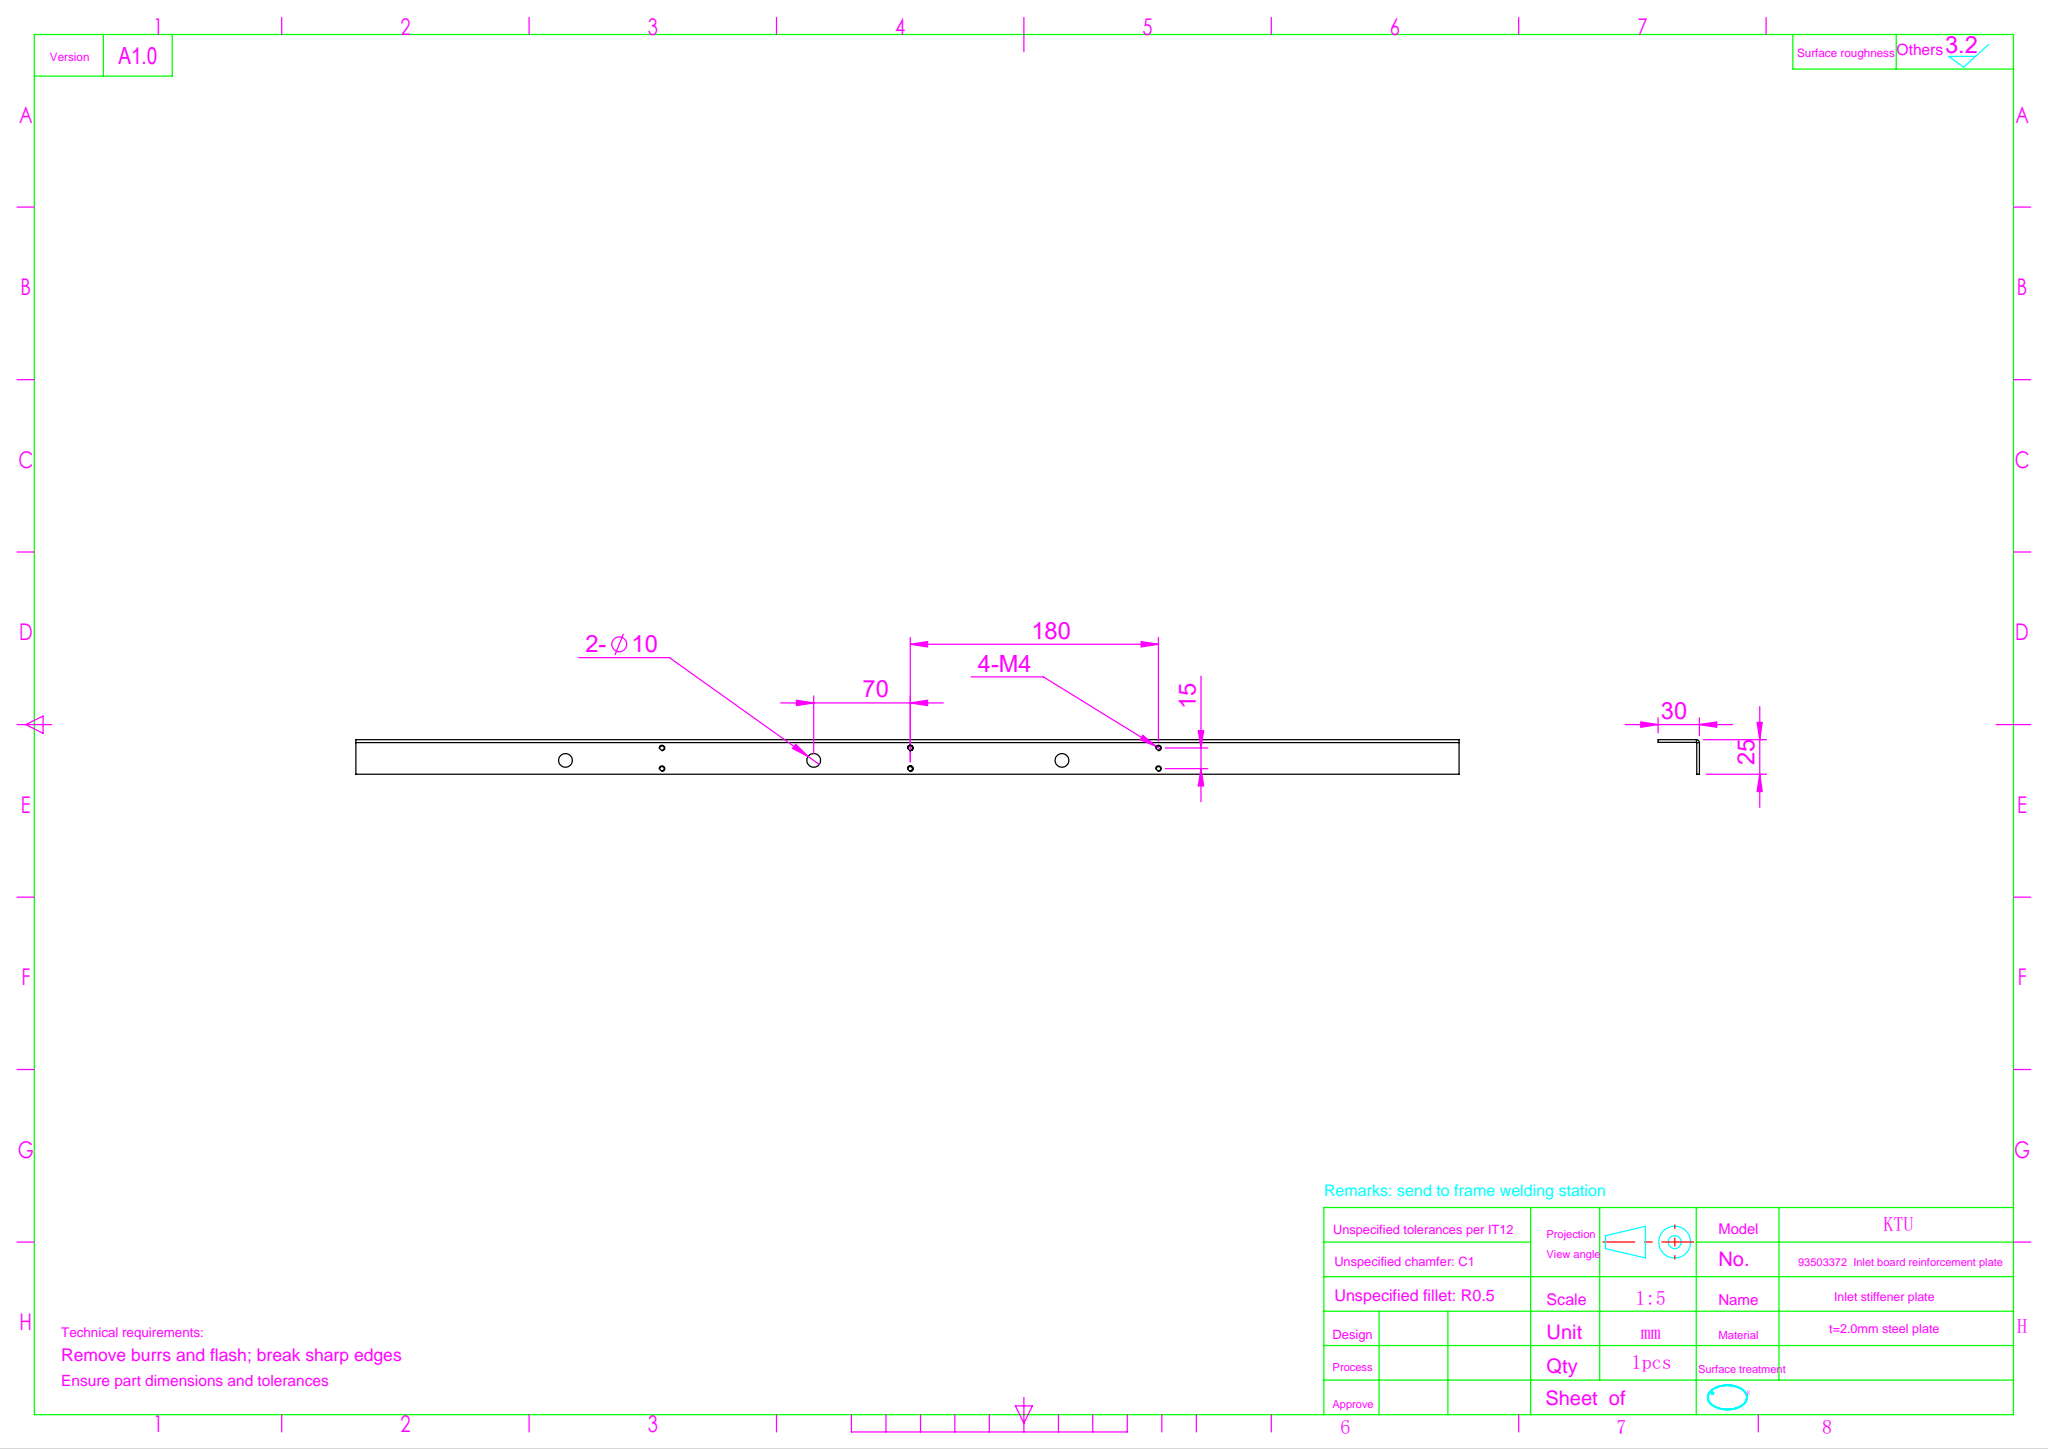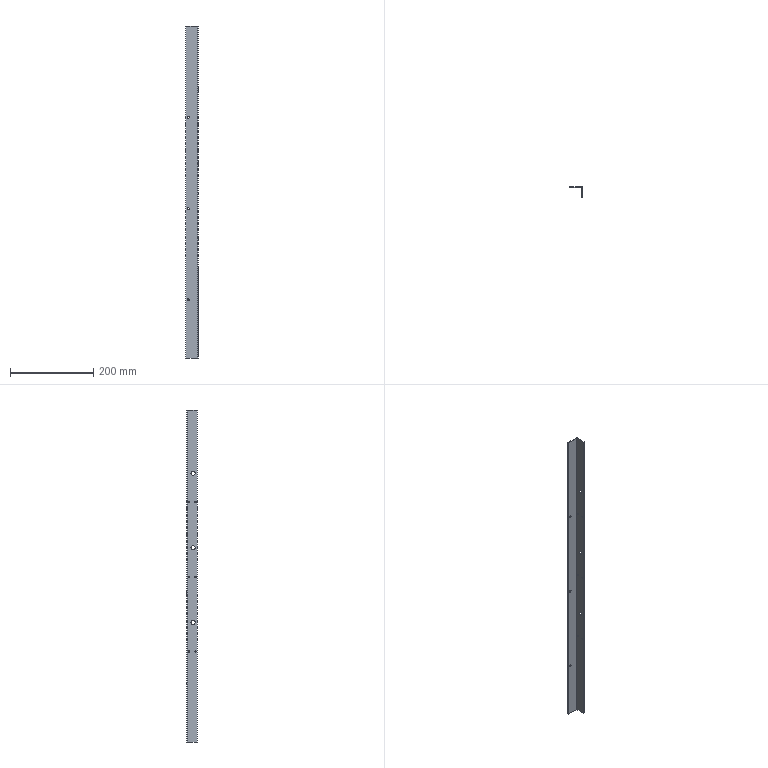Part | SolidWorks | features ICE 2, FlatPattern 1, LPattern 1, SMBaseFlange 1, SheetMetal 1 | 1 solid | 38 faces | box 30 x 25 x 800 mm | volume 83290 mm3 | cylinder 26 | plane 12 | commonest cylinder face diameters 3.2 x12 5 x6 10 x6 0.4 x1 4.4 x1